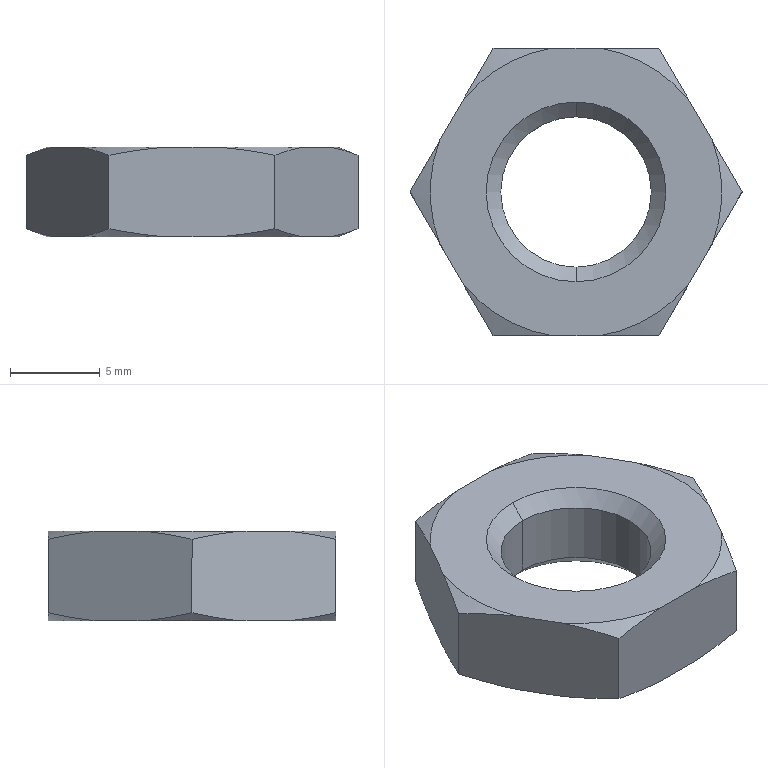Part | STEP file | Microwave Drying Flat Conveyor-nut_iso_4035_-_d_m10_-_05 | 1 solid | 26 faces | box 18.475 x 16 x 5 mm | volume 809.954 mm3 | cone 16 | plane 8 | cylinder 2 | commonest cylinder face diameters 8.376 x2
STEP:
#1=CARTESIAN_POINT('',(0.,-4.188,0.8119));
#2=VERTEX_POINT('',#1);
#3=CARTESIAN_POINT('',(0.,4.188,0.8119));
#4=VERTEX_POINT('',#3);
#5=CARTESIAN_POINT('',(0.,0.,0.8119));
#6=DIRECTION('',(0.,0.,-1.));
#7=DIRECTION('',(0.,1.,0.));
#8=AXIS2_PLACEMENT_3D('',#5,#6,#7);
#9=CIRCLE('',#8,4.188);
#10=EDGE_CURVE('',#2,#4,#9,.T.);
#11=ORIENTED_EDGE('',*,*,#10,.F.);
#12=CARTESIAN_POINT('',(0.,-5.,0.));
#13=VERTEX_POINT('',#12);
#14=CARTESIAN_POINT('',(0.,-4.188,0.8119));
#15=DIRECTION('',(0.,-0.7071,-0.7071));
#16=VECTOR('',#15,1000.);
#17=LINE('',#14,#16);
#18=EDGE_CURVE('',#2,#13,#17,.T.);
#19=ORIENTED_EDGE('',*,*,#18,.T.);
#20=CARTESIAN_POINT('',(0.,5.,0.));
#21=VERTEX_POINT('',#20);
#22=CARTESIAN_POINT('',(0.,0.,0.));
#23=DIRECTION('',(0.,0.,-1.));
#24=DIRECTION('',(1.,0.,0.));
#25=AXIS2_PLACEMENT_3D('',#22,#23,#24);
#26=CIRCLE('',#25,5.);
#27=EDGE_CURVE('',#13,#21,#26,.T.);
#28=ORIENTED_EDGE('',*,*,#27,.T.);
#29=CARTESIAN_POINT('',(0.,4.188,0.8119));
#30=DIRECTION('',(0.,0.7071,-0.7071));
#31=VECTOR('',#30,1000.);
#32=LINE('',#29,#31);
#33=EDGE_CURVE('',#4,#21,#32,.T.);
#34=ORIENTED_EDGE('',*,*,#33,.F.);
#35=EDGE_LOOP('',(#11,#19,#28,#34));
#36=FACE_OUTER_BOUND('',#35,.T.);
#37=CARTESIAN_POINT('',(0.,0.,0.8119));
#38=DIRECTION('',(0.,0.,-1.));
#39=DIRECTION('',(0.,1.,0.));
#40=AXIS2_PLACEMENT_3D('',#37,#38,#39);
#41=CONICAL_SURFACE('',#40,4.188,0.7854);
#42=ADVANCED_FACE('',(#36),#41,.F.);
#43=CARTESIAN_POINT('',(0.,-4.188,4.188));
#44=VERTEX_POINT('',#43);
#45=CARTESIAN_POINT('',(0.,4.188,4.188));
#46=VERTEX_POINT('',#45);
#47=CARTESIAN_POINT('',(0.,0.,4.188));
#48=DIRECTION('',(0.,0.,-1.));
#49=DIRECTION('',(0.,1.,0.));
#50=AXIS2_PLACEMENT_3D('',#47,#48,#49);
#51=CIRCLE('',#50,4.188);
#52=EDGE_CURVE('',#44,#46,#51,.T.);
#53=ORIENTED_EDGE('',*,*,#52,.F.);
#54=CARTESIAN_POINT('',(0.,-4.188,0.));
#55=DIRECTION('',(0.,0.,-1.));
#56=VECTOR('',#55,1000.);
#57=LINE('',#54,#56);
#58=EDGE_CURVE('',#44,#2,#57,.T.);
#59=ORIENTED_EDGE('',*,*,#58,.T.);
#60=ORIENTED_EDGE('',*,*,#10,.T.);
#61=CARTESIAN_POINT('',(0.,4.188,0.));
#62=DIRECTION('',(0.,0.,-1.));
#63=VECTOR('',#62,1000.);
#64=LINE('',#61,#63);
#65=EDGE_CURVE('',#46,#4,#64,.T.);
#66=ORIENTED_EDGE('',*,*,#65,.F.);
#67=EDGE_LOOP('',(#53,#59,#60,#66));
#68=FACE_OUTER_BOUND('',#67,.T.);
#69=CARTESIAN_POINT('',(0.,0.,0.));
#70=DIRECTION('',(0.,0.,-1.));
#71=DIRECTION('',(0.,1.,0.));
#72=AXIS2_PLACEMENT_3D('',#69,#70,#71);
#73=CYLINDRICAL_SURFACE('',#72,4.188);
#74=ADVANCED_FACE('',(#68),#73,.F.);
#75=ORIENTED_EDGE('',*,*,#52,.T.);
#76=CARTESIAN_POINT('',(0.,5.,5.));
#77=VERTEX_POINT('',#76);
#78=CARTESIAN_POINT('',(0.,5.,5.));
#79=DIRECTION('',(0.,0.7071,0.7071));
#80=VECTOR('',#79,1000.);
#81=LINE('',#78,#80);
#82=EDGE_CURVE('',#46,#77,#81,.T.);
#83=ORIENTED_EDGE('',*,*,#82,.T.);
#84=CARTESIAN_POINT('',(0.,-5.,5.));
#85=VERTEX_POINT('',#84);
#86=CARTESIAN_POINT('',(0.,0.,5.));
#87=DIRECTION('',(0.,0.,-1.));
#88=DIRECTION('',(0.,1.,0.));
#89=AXIS2_PLACEMENT_3D('',#86,#87,#88);
#90=CIRCLE('',#89,5.);
#91=EDGE_CURVE('',#85,#77,#90,.T.);
#92=ORIENTED_EDGE('',*,*,#91,.F.);
#93=CARTESIAN_POINT('',(0.,-5.,5.));
#94=DIRECTION('',(0.,-0.7071,0.7071));
#95=VECTOR('',#94,1000.);
#96=LINE('',#93,#95);
#97=EDGE_CURVE('',#44,#85,#96,.T.);
#98=ORIENTED_EDGE('',*,*,#97,.F.);
#99=EDGE_LOOP('',(#75,#83,#92,#98));
#100=FACE_OUTER_BOUND('',#99,.T.);
#101=CARTESIAN_POINT('',(0.,0.,5.));
#102=DIRECTION('',(0.,0.,1.));
#103=DIRECTION('',(0.,-1.,0.));
#104=AXIS2_PLACEMENT_3D('',#101,#102,#103);
#105=CONICAL_SURFACE('',#104,5.,0.7854);
#106=ADVANCED_FACE('',(#100),#105,.F.);
#107=CARTESIAN_POINT('',(7.602,2.834,0.));
#108=VERTEX_POINT('',#107);
#109=CARTESIAN_POINT('',(9.238,0.,0.4545));
#110=VERTEX_POINT('',#109);
#111=CARTESIAN_POINT('',(7.602,2.834,0.));
#112=CARTESIAN_POINT('',(8.152,1.88,0.07388));
#113=CARTESIAN_POINT('',(8.697,0.9365,0.2361));
#114=CARTESIAN_POINT('',(9.238,0.,0.4545));
#115=B_SPLINE_CURVE_WITH_KNOTS('',3,(#111,#112,#113,#114),.UNSPECIFIED.,.F.,.F.,(4,4),(0.00000003,0.003304),.UNSPECIFIED.);
#116=EDGE_CURVE('',#108,#110,#115,.T.);
#117=ORIENTED_EDGE('',*,*,#116,.T.);
#118=CARTESIAN_POINT('',(7.602,-2.834,0.));
#119=VERTEX_POINT('',#118);
#120=CARTESIAN_POINT('',(9.238,0.,0.4545));
#121=CARTESIAN_POINT('',(8.697,-0.9365,0.2361));
#122=CARTESIAN_POINT('',(8.152,-1.88,0.07388));
#123=CARTESIAN_POINT('',(7.602,-2.834,0.));
#124=B_SPLINE_CURVE_WITH_KNOTS('',3,(#120,#121,#122,#123),.UNSPECIFIED.,.F.,.F.,(4,4),(0.000000002,0.003303),.UNSPECIFIED.);
#125=EDGE_CURVE('',#110,#119,#124,.T.);
#126=ORIENTED_EDGE('',*,*,#125,.T.);
#127=CARTESIAN_POINT('',(0.,0.,0.));
#128=DIRECTION('',(0.,0.,1.));
#129=DIRECTION('',(1.,0.,0.));
#130=AXIS2_PLACEMENT_3D('',#127,#128,#129);
#131=CIRCLE('',#130,8.113);
#132=EDGE_CURVE('',#119,#108,#131,.T.);
#133=ORIENTED_EDGE('',*,*,#132,.T.);
#134=EDGE_LOOP('',(#117,#126,#133));
#135=FACE_OUTER_BOUND('',#134,.T.);
#136=CARTESIAN_POINT('',(0.,0.,0.));
#137=DIRECTION('',(0.,0.,1.));
#138=DIRECTION('',(0.,-1.,0.));
#139=AXIS2_PLACEMENT_3D('',#136,#137,#138);
#140=CONICAL_SURFACE('',#139,8.113,1.187);
#141=ADVANCED_FACE('',(#135),#140,.T.);
#142=CARTESIAN_POINT('',(6.255,-5.166,0.));
#143=VERTEX_POINT('',#142);
#144=CARTESIAN_POINT('',(4.619,-8.,0.4545));
#145=VERTEX_POINT('',#144);
#146=CARTESIAN_POINT('',(6.255,-5.166,0.));
#147=CARTESIAN_POINT('',(5.704,-6.12,0.07388));
#148=CARTESIAN_POINT('',(5.159,-7.063,0.2361));
#149=CARTESIAN_POINT('',(4.619,-8.,0.4545));
#150=B_SPLINE_CURVE_WITH_KNOTS('',3,(#146,#147,#148,#149),.UNSPECIFIED.,.F.,.F.,(4,4),(0.00000003,0.003304),.UNSPECIFIED.);
#151=EDGE_CURVE('',#143,#145,#150,.T.);
#152=ORIENTED_EDGE('',*,*,#151,.F.);
#153=CARTESIAN_POINT('',(4.619,-8.,0.));
#154=DIRECTION('',(0.5,0.866,0.));
#155=VECTOR('',#154,1000.);
#156=LINE('',#153,#155);
#157=EDGE_CURVE('',#143,#119,#156,.T.);
#158=ORIENTED_EDGE('',*,*,#157,.T.);
#159=ORIENTED_EDGE('',*,*,#125,.F.);
#160=CARTESIAN_POINT('',(9.238,0.,4.545));
#161=VERTEX_POINT('',#160);
#162=CARTESIAN_POINT('',(9.238,0.,5.));
#163=DIRECTION('',(0.,0.,-1.));
#164=VECTOR('',#163,1000.);
#165=LINE('',#162,#164);
#166=EDGE_CURVE('',#161,#110,#165,.T.);
#167=ORIENTED_EDGE('',*,*,#166,.F.);
#168=CARTESIAN_POINT('',(7.602,-2.834,5.));
#169=VERTEX_POINT('',#168);
#170=CARTESIAN_POINT('',(7.602,-2.834,5.));
#171=CARTESIAN_POINT('',(8.152,-1.88,4.926));
#172=CARTESIAN_POINT('',(8.697,-0.9365,4.764));
#173=CARTESIAN_POINT('',(9.238,0.,4.545));
#174=B_SPLINE_CURVE_WITH_KNOTS('',3,(#170,#171,#172,#173),.UNSPECIFIED.,.F.,.F.,(4,4),(0.00000003,0.003304),.UNSPECIFIED.);
#175=EDGE_CURVE('',#169,#161,#174,.T.);
#176=ORIENTED_EDGE('',*,*,#175,.F.);
#177=CARTESIAN_POINT('',(6.255,-5.166,5.));
#178=VERTEX_POINT('',#177);
#179=CARTESIAN_POINT('',(4.619,-8.,5.));
#180=DIRECTION('',(0.5,0.866,0.));
#181=VECTOR('',#180,1000.);
#182=LINE('',#179,#181);
#183=EDGE_CURVE('',#178,#169,#182,.T.);
#184=ORIENTED_EDGE('',*,*,#183,.F.);
#185=CARTESIAN_POINT('',(4.619,-8.,4.545));
#186=VERTEX_POINT('',#185);
#187=CARTESIAN_POINT('',(4.619,-8.,4.545));
#188=CARTESIAN_POINT('',(5.159,-7.063,4.764));
#189=CARTESIAN_POINT('',(5.704,-6.12,4.926));
#190=CARTESIAN_POINT('',(6.255,-5.166,5.));
#191=B_SPLINE_CURVE_WITH_KNOTS('',3,(#187,#188,#189,#190),.UNSPECIFIED.,.F.,.F.,(4,4),(0.000000002,0.003303),.UNSPECIFIED.);
#192=EDGE_CURVE('',#186,#178,#191,.T.);
#193=ORIENTED_EDGE('',*,*,#192,.F.);
#194=CARTESIAN_POINT('',(4.619,-8.,5.));
#195=DIRECTION('',(0.,0.,-1.));
#196=VECTOR('',#195,1000.);
#197=LINE('',#194,#196);
#198=EDGE_CURVE('',#186,#145,#197,.T.);
#199=ORIENTED_EDGE('',*,*,#198,.T.);
#200=EDGE_LOOP('',(#152,#158,#159,#167,#176,#184,#193,#199));
#201=FACE_OUTER_BOUND('',#200,.T.);
#202=CARTESIAN_POINT('',(4.619,-8.,5.));
#203=DIRECTION('',(-0.866,0.5,0.));
#204=DIRECTION('',(-0.5,-0.866,0.));
#205=AXIS2_PLACEMENT_3D('',#202,#203,#204);
#206=PLANE('',#205);
#207=ADVANCED_FACE('',(#201),#206,.F.);
#208=ORIENTED_EDGE('',*,*,#116,.F.);
#209=CARTESIAN_POINT('',(6.255,5.166,0.));
#210=VERTEX_POINT('',#209);
#211=CARTESIAN_POINT('',(9.238,0.,0.));
#212=DIRECTION('',(-0.5,0.866,0.));
#213=VECTOR('',#212,1000.);
#214=LINE('',#211,#213);
#215=EDGE_CURVE('',#108,#210,#214,.T.);
#216=ORIENTED_EDGE('',*,*,#215,.T.);
#217=CARTESIAN_POINT('',(4.619,8.,0.4545));
#218=VERTEX_POINT('',#217);
#219=CARTESIAN_POINT('',(4.619,8.,0.4545));
#220=CARTESIAN_POINT('',(5.159,7.063,0.2361));
#221=CARTESIAN_POINT('',(5.704,6.12,0.07388));
#222=CARTESIAN_POINT('',(6.255,5.166,0.));
#223=B_SPLINE_CURVE_WITH_KNOTS('',3,(#219,#220,#221,#222),.UNSPECIFIED.,.F.,.F.,(4,4),(0.000000002,0.003303),.UNSPECIFIED.);
#224=EDGE_CURVE('',#218,#210,#223,.T.);
#225=ORIENTED_EDGE('',*,*,#224,.F.);
#226=CARTESIAN_POINT('',(4.619,8.,4.545));
#227=VERTEX_POINT('',#226);
#228=CARTESIAN_POINT('',(4.619,8.,5.));
#229=DIRECTION('',(0.,0.,-1.));
#230=VECTOR('',#229,1000.);
#231=LINE('',#228,#230);
#232=EDGE_CURVE('',#227,#218,#231,.T.);
#233=ORIENTED_EDGE('',*,*,#232,.F.);
#234=CARTESIAN_POINT('',(6.255,5.166,5.));
#235=VERTEX_POINT('',#234);
#236=CARTESIAN_POINT('',(6.255,5.166,5.));
#237=CARTESIAN_POINT('',(5.704,6.12,4.926));
#238=CARTESIAN_POINT('',(5.159,7.063,4.764));
#239=CARTESIAN_POINT('',(4.619,8.,4.545));
#240=B_SPLINE_CURVE_WITH_KNOTS('',3,(#236,#237,#238,#239),.UNSPECIFIED.,.F.,.F.,(4,4),(0.00000003,0.003304),.UNSPECIFIED.);
#241=EDGE_CURVE('',#235,#227,#240,.T.);
#242=ORIENTED_EDGE('',*,*,#241,.F.);
#243=CARTESIAN_POINT('',(7.602,2.834,5.));
#244=VERTEX_POINT('',#243);
#245=CARTESIAN_POINT('',(9.238,0.,5.));
#246=DIRECTION('',(-0.5,0.866,0.));
#247=VECTOR('',#246,1000.);
#248=LINE('',#245,#247);
#249=EDGE_CURVE('',#244,#235,#248,.T.);
#250=ORIENTED_EDGE('',*,*,#249,.F.);
#251=CARTESIAN_POINT('',(9.238,0.,4.545));
#252=CARTESIAN_POINT('',(8.697,0.9365,4.764));
#253=CARTESIAN_POINT('',(8.152,1.88,4.926));
#254=CARTESIAN_POINT('',(7.602,2.834,5.));
#255=B_SPLINE_CURVE_WITH_KNOTS('',3,(#251,#252,#253,#254),.UNSPECIFIED.,.F.,.F.,(4,4),(0.000000002,0.003303),.UNSPECIFIED.);
#256=EDGE_CURVE('',#161,#244,#255,.T.);
#257=ORIENTED_EDGE('',*,*,#256,.F.);
#258=ORIENTED_EDGE('',*,*,#166,.T.);
#259=EDGE_LOOP('',(#208,#216,#225,#233,#242,#250,#257,#258));
#260=FACE_OUTER_BOUND('',#259,.T.);
#261=CARTESIAN_POINT('',(9.238,0.,5.));
#262=DIRECTION('',(-0.866,-0.5,0.));
#263=DIRECTION('',(0.5,-0.866,0.));
#264=AXIS2_PLACEMENT_3D('',#261,#262,#263);
#265=PLANE('',#264);
#266=ADVANCED_FACE('',(#260),#265,.F.);
#267=CARTESIAN_POINT('',(-4.619,8.,0.4545));
#268=VERTEX_POINT('',#267);
#269=CARTESIAN_POINT('',(-1.347,8.,0.));
#270=VERTEX_POINT('',#269);
#271=CARTESIAN_POINT('',(-4.619,8.,0.4545));
#272=CARTESIAN_POINT('',(-4.078,8.,0.3453));
#273=CARTESIAN_POINT('',(-3.532,8.,0.2495));
#274=CARTESIAN_POINT('',(-2.439,8.,0.0951));
#275=CARTESIAN_POINT('',(-1.893,8.,0.03663));
#276=CARTESIAN_POINT('',(-1.347,8.,0.));
#277=B_SPLINE_CURVE_WITH_KNOTS('',3,(#271,#272,#273,#274,#275,#276),.UNSPECIFIED.,.F.,.F.,(4,2,4),(0.007925,0.009576,0.01123),.UNSPECIFIED.);
#278=EDGE_CURVE('',#268,#270,#277,.T.);
#279=ORIENTED_EDGE('',*,*,#278,.F.);
#280=CARTESIAN_POINT('',(-4.619,8.,4.545));
#281=VERTEX_POINT('',#280);
#282=CARTESIAN_POINT('',(-4.619,8.,5.));
#283=DIRECTION('',(0.,0.,-1.));
#284=VECTOR('',#283,1000.);
#285=LINE('',#282,#284);
#286=EDGE_CURVE('',#281,#268,#285,.T.);
#287=ORIENTED_EDGE('',*,*,#286,.F.);
#288=CARTESIAN_POINT('',(-1.347,8.,5.));
#289=VERTEX_POINT('',#288);
#290=CARTESIAN_POINT('',(-1.347,8.,5.));
#291=CARTESIAN_POINT('',(-1.893,8.,4.963));
#292=CARTESIAN_POINT('',(-2.439,8.,4.905));
#293=CARTESIAN_POINT('',(-3.532,8.,4.751));
#294=CARTESIAN_POINT('',(-4.078,8.,4.655));
#295=CARTESIAN_POINT('',(-4.619,8.,4.545));
#296=B_SPLINE_CURVE_WITH_KNOTS('',3,(#290,#291,#292,#293,#294,#295),.UNSPECIFIED.,.F.,.F.,(4,2,4),(0.02193,0.02357,0.02522),.UNSPECIFIED.);
#297=EDGE_CURVE('',#289,#281,#296,.T.);
#298=ORIENTED_EDGE('',*,*,#297,.F.);
#299=CARTESIAN_POINT('',(1.347,8.,5.));
#300=VERTEX_POINT('',#299);
#301=CARTESIAN_POINT('',(4.619,8.,5.));
#302=DIRECTION('',(-1.,0.,0.));
#303=VECTOR('',#302,1000.);
#304=LINE('',#301,#303);
#305=EDGE_CURVE('',#300,#289,#304,.T.);
#306=ORIENTED_EDGE('',*,*,#305,.F.);
#307=CARTESIAN_POINT('',(4.619,8.,4.545));
#308=CARTESIAN_POINT('',(4.078,8.,4.655));
#309=CARTESIAN_POINT('',(3.531,8.,4.751));
#310=CARTESIAN_POINT('',(2.439,8.,4.905));
#311=CARTESIAN_POINT('',(1.893,8.,4.963));
#312=CARTESIAN_POINT('',(1.347,8.,5.));
#313=B_SPLINE_CURVE_WITH_KNOTS('',3,(#307,#308,#309,#310,#311,#312),.UNSPECIFIED.,.F.,.F.,(4,2,4),(0.01593,0.01758,0.01922),.UNSPECIFIED.);
#314=EDGE_CURVE('',#227,#300,#313,.T.);
#315=ORIENTED_EDGE('',*,*,#314,.F.);
#316=ORIENTED_EDGE('',*,*,#232,.T.);
#317=CARTESIAN_POINT('',(1.347,8.,0.));
#318=VERTEX_POINT('',#317);
#319=CARTESIAN_POINT('',(1.347,8.,0.));
#320=CARTESIAN_POINT('',(1.893,8.,0.03664));
#321=CARTESIAN_POINT('',(2.439,8.,0.09509));
#322=CARTESIAN_POINT('',(3.531,8.,0.2494));
#323=CARTESIAN_POINT('',(4.078,8.,0.3453));
#324=CARTESIAN_POINT('',(4.619,8.,0.4545));
#325=B_SPLINE_CURVE_WITH_KNOTS('',3,(#319,#320,#321,#322,#323,#324),.UNSPECIFIED.,.F.,.F.,(4,2,4),(0.01394,0.0156,0.01725),.UNSPECIFIED.);
#326=EDGE_CURVE('',#318,#218,#325,.T.);
#327=ORIENTED_EDGE('',*,*,#326,.F.);
#328=CARTESIAN_POINT('',(4.619,8.,0.));
#329=DIRECTION('',(-1.,0.,0.));
#330=VECTOR('',#329,1000.);
#331=LINE('',#328,#330);
#332=EDGE_CURVE('',#318,#270,#331,.T.);
#333=ORIENTED_EDGE('',*,*,#332,.T.);
#334=EDGE_LOOP('',(#279,#287,#298,#306,#315,#316,#327,#333));
#335=FACE_OUTER_BOUND('',#334,.T.);
#336=CARTESIAN_POINT('',(4.619,8.,5.));
#337=DIRECTION('',(0.,-1.,0.));
#338=DIRECTION('',(1.,0.,0.));
#339=AXIS2_PLACEMENT_3D('',#336,#337,#338);
#340=PLANE('',#339);
#341=ADVANCED_FACE('',(#335),#340,.F.);
#342=CARTESIAN_POINT('',(-6.255,5.166,0.));
#343=VERTEX_POINT('',#342);
#344=CARTESIAN_POINT('',(-6.255,5.166,0.));
#345=CARTESIAN_POINT('',(-5.704,6.12,0.07388));
#346=CARTESIAN_POINT('',(-5.159,7.063,0.2361));
#347=CARTESIAN_POINT('',(-4.619,8.,0.4545));
#348=B_SPLINE_CURVE_WITH_KNOTS('',3,(#344,#345,#346,#347),.UNSPECIFIED.,.F.,.F.,(4,4),(0.00000003,0.003304),.UNSPECIFIED.);
#349=EDGE_CURVE('',#343,#268,#348,.T.);
#350=ORIENTED_EDGE('',*,*,#349,.F.);
#351=CARTESIAN_POINT('',(-7.602,2.834,0.));
#352=VERTEX_POINT('',#351);
#353=CARTESIAN_POINT('',(-4.619,8.,0.));
#354=DIRECTION('',(-0.5,-0.866,0.));
#355=VECTOR('',#354,1000.);
#356=LINE('',#353,#355);
#357=EDGE_CURVE('',#343,#352,#356,.T.);
#358=ORIENTED_EDGE('',*,*,#357,.T.);
#359=CARTESIAN_POINT('',(-9.238,0.,0.4545));
#360=VERTEX_POINT('',#359);
#361=CARTESIAN_POINT('',(-9.238,0.,0.4545));
#362=CARTESIAN_POINT('',(-8.697,0.9365,0.2361));
#363=CARTESIAN_POINT('',(-8.152,1.88,0.07388));
#364=CARTESIAN_POINT('',(-7.602,2.834,0.));
#365=B_SPLINE_CURVE_WITH_KNOTS('',3,(#361,#362,#363,#364),.UNSPECIFIED.,.F.,.F.,(4,4),(0.000000002,0.003303),.UNSPECIFIED.);
#366=EDGE_CURVE('',#360,#352,#365,.T.);
#367=ORIENTED_EDGE('',*,*,#366,.F.);
#368=CARTESIAN_POINT('',(-9.238,0.,4.545));
#369=VERTEX_POINT('',#368);
#370=CARTESIAN_POINT('',(-9.238,0.,5.));
#371=DIRECTION('',(0.,0.,-1.));
#372=VECTOR('',#371,1000.);
#373=LINE('',#370,#372);
#374=EDGE_CURVE('',#369,#360,#373,.T.);
#375=ORIENTED_EDGE('',*,*,#374,.F.);
#376=CARTESIAN_POINT('',(-7.602,2.834,5.));
#377=VERTEX_POINT('',#376);
#378=CARTESIAN_POINT('',(-7.602,2.834,5.));
#379=CARTESIAN_POINT('',(-8.152,1.88,4.926));
#380=CARTESIAN_POINT('',(-8.697,0.9365,4.764));
#381=CARTESIAN_POINT('',(-9.238,0.,4.545));
#382=B_SPLINE_CURVE_WITH_KNOTS('',3,(#378,#379,#380,#381),.UNSPECIFIED.,.F.,.F.,(4,4),(0.00000003,0.003304),.UNSPECIFIED.);
#383=EDGE_CURVE('',#377,#369,#382,.T.);
#384=ORIENTED_EDGE('',*,*,#383,.F.);
#385=CARTESIAN_POINT('',(-6.255,5.166,5.));
#386=VERTEX_POINT('',#385);
#387=CARTESIAN_POINT('',(-4.619,8.,5.));
#388=DIRECTION('',(-0.5,-0.866,0.));
#389=VECTOR('',#388,1000.);
#390=LINE('',#387,#389);
#391=EDGE_CURVE('',#386,#377,#390,.T.);
#392=ORIENTED_EDGE('',*,*,#391,.F.);
#393=CARTESIAN_POINT('',(-4.619,8.,4.545));
#394=CARTESIAN_POINT('',(-5.159,7.063,4.764));
#395=CARTESIAN_POINT('',(-5.704,6.12,4.926));
#396=CARTESIAN_POINT('',(-6.255,5.166,5.));
#397=B_SPLINE_CURVE_WITH_KNOTS('',3,(#393,#394,#395,#396),.UNSPECIFIED.,.F.,.F.,(4,4),(0.000000002,0.003303),.UNSPECIFIED.);
#398=EDGE_CURVE('',#281,#386,#397,.T.);
#399=ORIENTED_EDGE('',*,*,#398,.F.);
#400=ORIENTED_EDGE('',*,*,#286,.T.);
#401=EDGE_LOOP('',(#350,#358,#367,#375,#384,#392,#399,#400));
#402=FACE_OUTER_BOUND('',#401,.T.);
#403=CARTESIAN_POINT('',(-4.619,8.,5.));
#404=DIRECTION('',(0.866,-0.5,0.));
#405=DIRECTION('',(0.5,0.866,0.));
#406=AXIS2_PLACEMENT_3D('',#403,#404,#405);
#407=PLANE('',#406);
#408=ADVANCED_FACE('',(#402),#407,.F.);
#409=CARTESIAN_POINT('',(-7.602,-2.834,0.));
#410=VERTEX_POINT('',#409);
#411=CARTESIAN_POINT('',(-7.602,-2.834,0.));
#412=CARTESIAN_POINT('',(-8.152,-1.88,0.07388));
#413=CARTESIAN_POINT('',(-8.697,-0.9365,0.2361));
#414=CARTESIAN_POINT('',(-9.238,0.,0.4545));
#415=B_SPLINE_CURVE_WITH_KNOTS('',3,(#411,#412,#413,#414),.UNSPECIFIED.,.F.,.F.,(4,4),(0.00000003,0.003304),.UNSPECIFIED.);
#416=EDGE_CURVE('',#410,#360,#415,.T.);
#417=ORIENTED_EDGE('',*,*,#416,.F.);
#418=CARTESIAN_POINT('',(-6.255,-5.166,0.));
#419=VERTEX_POINT('',#418);
#420=CARTESIAN_POINT('',(-9.238,0.,0.));
#421=DIRECTION('',(0.5,-0.866,0.));
#422=VECTOR('',#421,1000.);
#423=LINE('',#420,#422);
#424=EDGE_CURVE('',#410,#419,#423,.T.);
#425=ORIENTED_EDGE('',*,*,#424,.T.);
#426=CARTESIAN_POINT('',(-4.619,-8.,0.4545));
#427=VERTEX_POINT('',#426);
#428=CARTESIAN_POINT('',(-4.619,-8.,0.4545));
#429=CARTESIAN_POINT('',(-5.159,-7.063,0.2361));
#430=CARTESIAN_POINT('',(-5.704,-6.12,0.07388));
#431=CARTESIAN_POINT('',(-6.255,-5.166,0.));
#432=B_SPLINE_CURVE_WITH_KNOTS('',3,(#428,#429,#430,#431),.UNSPECIFIED.,.F.,.F.,(4,4),(0.000000002,0.003303),.UNSPECIFIED.);
#433=EDGE_CURVE('',#427,#419,#432,.T.);
#434=ORIENTED_EDGE('',*,*,#433,.F.);
#435=CARTESIAN_POINT('',(-4.619,-8.,4.545));
#436=VERTEX_POINT('',#435);
#437=CARTESIAN_POINT('',(-4.619,-8.,5.));
#438=DIRECTION('',(0.,0.,-1.));
#439=VECTOR('',#438,1000.);
#440=LINE('',#437,#439);
#441=EDGE_CURVE('',#436,#427,#440,.T.);
#442=ORIENTED_EDGE('',*,*,#441,.F.);
#443=CARTESIAN_POINT('',(-6.255,-5.166,5.));
#444=VERTEX_POINT('',#443);
#445=CARTESIAN_POINT('',(-6.255,-5.166,5.));
#446=CARTESIAN_POINT('',(-5.704,-6.12,4.926));
#447=CARTESIAN_POINT('',(-5.159,-7.063,4.764));
#448=CARTESIAN_POINT('',(-4.619,-8.,4.545));
#449=B_SPLINE_CURVE_WITH_KNOTS('',3,(#445,#446,#447,#448),.UNSPECIFIED.,.F.,.F.,(4,4),(0.00000003,0.003304),.UNSPECIFIED.);
#450=EDGE_CURVE('',#444,#436,#449,.T.);
#451=ORIENTED_EDGE('',*,*,#450,.F.);
#452=CARTESIAN_POINT('',(-7.602,-2.834,5.));
#453=VERTEX_POINT('',#452);
#454=CARTESIAN_POINT('',(-9.238,0.,5.));
#455=DIRECTION('',(0.5,-0.866,0.));
#456=VECTOR('',#455,1000.);
#457=LINE('',#454,#456);
#458=EDGE_CURVE('',#453,#444,#457,.T.);
#459=ORIENTED_EDGE('',*,*,#458,.F.);
#460=CARTESIAN_POINT('',(-9.238,0.,4.545));
#461=CARTESIAN_POINT('',(-8.697,-0.9365,4.764));
#462=CARTESIAN_POINT('',(-8.152,-1.88,4.926));
#463=CARTESIAN_POINT('',(-7.602,-2.834,5.));
#464=B_SPLINE_CURVE_WITH_KNOTS('',3,(#460,#461,#462,#463),.UNSPECIFIED.,.F.,.F.,(4,4),(0.000000002,0.003303),.UNSPECIFIED.);
#465=EDGE_CURVE('',#369,#453,#464,.T.);
#466=ORIENTED_EDGE('',*,*,#465,.F.);
#467=ORIENTED_EDGE('',*,*,#374,.T.);
#468=EDGE_LOOP('',(#417,#425,#434,#442,#451,#459,#466,#467));
#469=FACE_OUTER_BOUND('',#468,.T.);
#470=CARTESIAN_POINT('',(-9.238,0.,5.));
#471=DIRECTION('',(0.866,0.5,0.));
#472=DIRECTION('',(-0.5,0.866,0.));
#473=AXIS2_PLACEMENT_3D('',#470,#471,#472);
#474=PLANE('',#473);
#475=ADVANCED_FACE('',(#469),#474,.F.);
#476=CARTESIAN_POINT('',(1.347,-8.,0.));
#477=VERTEX_POINT('',#476);
#478=CARTESIAN_POINT('',(4.619,-8.,0.4545));
#479=CARTESIAN_POINT('',(4.078,-8.,0.3453));
#480=CARTESIAN_POINT('',(3.531,-8.,0.2494));
#481=CARTESIAN_POINT('',(2.439,-8.,0.09509));
#482=CARTESIAN_POINT('',(1.893,-8.,0.03664));
#483=CARTESIAN_POINT('',(1.347,-8.,0.));
#484=B_SPLINE_CURVE_WITH_KNOTS('',3,(#478,#479,#480,#481,#482,#483),.UNSPECIFIED.,.F.,.F.,(4,2,4),(0.01593,0.01758,0.01922),.UNSPECIFIED.);
#485=EDGE_CURVE('',#145,#477,#484,.T.);
#486=ORIENTED_EDGE('',*,*,#485,.F.);
#487=ORIENTED_EDGE('',*,*,#198,.F.);
#488=CARTESIAN_POINT('',(1.347,-8.,5.));
#489=VERTEX_POINT('',#488);
#490=CARTESIAN_POINT('',(1.347,-8.,5.));
#491=CARTESIAN_POINT('',(1.893,-8.,4.963));
#492=CARTESIAN_POINT('',(2.439,-8.,4.905));
#493=CARTESIAN_POINT('',(3.531,-8.,4.751));
#494=CARTESIAN_POINT('',(4.078,-8.,4.655));
#495=CARTESIAN_POINT('',(4.619,-8.,4.545));
#496=B_SPLINE_CURVE_WITH_KNOTS('',3,(#490,#491,#492,#493,#494,#495),.UNSPECIFIED.,.F.,.F.,(4,2,4),(0.01394,0.0156,0.01725),.UNSPECIFIED.);
#497=EDGE_CURVE('',#489,#186,#496,.T.);
#498=ORIENTED_EDGE('',*,*,#497,.F.);
#499=CARTESIAN_POINT('',(-1.347,-8.,5.));
#500=VERTEX_POINT('',#499);
#501=CARTESIAN_POINT('',(-4.619,-8.,5.));
#502=DIRECTION('',(1.,0.,0.));
#503=VECTOR('',#502,1000.);
#504=LINE('',#501,#503);
#505=EDGE_CURVE('',#500,#489,#504,.T.);
#506=ORIENTED_EDGE('',*,*,#505,.F.);
#507=CARTESIAN_POINT('',(-4.619,-8.,4.545));
#508=CARTESIAN_POINT('',(-4.078,-8.,4.655));
#509=CARTESIAN_POINT('',(-3.532,-8.,4.751));
#510=CARTESIAN_POINT('',(-2.439,-8.,4.905));
#511=CARTESIAN_POINT('',(-1.893,-8.,4.963));
#512=CARTESIAN_POINT('',(-1.347,-8.,5.));
#513=B_SPLINE_CURVE_WITH_KNOTS('',3,(#507,#508,#509,#510,#511,#512),.UNSPECIFIED.,.F.,.F.,(4,2,4),(0.007925,0.009576,0.01123),.UNSPECIFIED.);
#514=EDGE_CURVE('',#436,#500,#513,.T.);
#515=ORIENTED_EDGE('',*,*,#514,.F.);
#516=ORIENTED_EDGE('',*,*,#441,.T.);
#517=CARTESIAN_POINT('',(-1.347,-8.,0.));
#518=VERTEX_POINT('',#517);
#519=CARTESIAN_POINT('',(-1.347,-8.,0.));
#520=CARTESIAN_POINT('',(-1.893,-8.,0.03663));
#521=CARTESIAN_POINT('',(-2.439,-8.,0.0951));
#522=CARTESIAN_POINT('',(-3.532,-8.,0.2495));
#523=CARTESIAN_POINT('',(-4.078,-8.,0.3453));
#524=CARTESIAN_POINT('',(-4.619,-8.,0.4545));
#525=B_SPLINE_CURVE_WITH_KNOTS('',3,(#519,#520,#521,#522,#523,#524),.UNSPECIFIED.,.F.,.F.,(4,2,4),(0.02193,0.02357,0.02522),.UNSPECIFIED.);
#526=EDGE_CURVE('',#518,#427,#525,.T.);
#527=ORIENTED_EDGE('',*,*,#526,.F.);
#528=CARTESIAN_POINT('',(-4.619,-8.,0.));
#529=DIRECTION('',(1.,0.,0.));
#530=VECTOR('',#529,1000.);
#531=LINE('',#528,#530);
#532=EDGE_CURVE('',#518,#477,#531,.T.);
#533=ORIENTED_EDGE('',*,*,#532,.T.);
#534=EDGE_LOOP('',(#486,#487,#498,#506,#515,#516,#527,#533));
#535=FACE_OUTER_BOUND('',#534,.T.);
#536=CARTESIAN_POINT('',(-4.619,-8.,5.));
#537=DIRECTION('',(0.,1.,0.));
#538=DIRECTION('',(-1.,0.,0.));
#539=AXIS2_PLACEMENT_3D('',#536,#537,#538);
#540=PLANE('',#539);
#541=ADVANCED_FACE('',(#535),#540,.F.);
#542=ORIENTED_EDGE('',*,*,#91,.T.);
#543=CARTESIAN_POINT('',(0.,0.,5.));
#544=DIRECTION('',(0.,0.,-1.));
#545=DIRECTION('',(0.,1.,0.));
#546=AXIS2_PLACEMENT_3D('',#543,#544,#545);
#547=CIRCLE('',#546,5.);
#548=EDGE_CURVE('',#77,#85,#547,.T.);
#549=ORIENTED_EDGE('',*,*,#548,.T.);
#550=EDGE_LOOP('',(#542,#549));
#551=FACE_BOUND('',#550,.T.);
#552=ORIENTED_EDGE('',*,*,#249,.T.);
#553=CARTESIAN_POINT('',(0.,0.,5.));
#554=DIRECTION('',(0.,0.,-1.));
#555=DIRECTION('',(0.,1.,0.));
#556=AXIS2_PLACEMENT_3D('',#553,#554,#555);
#557=CIRCLE('',#556,8.113);
#558=EDGE_CURVE('',#300,#235,#557,.T.);
#559=ORIENTED_EDGE('',*,*,#558,.F.);
#560=ORIENTED_EDGE('',*,*,#305,.T.);
#561=CARTESIAN_POINT('',(0.,0.,5.));
#562=DIRECTION('',(0.,0.,1.));
#563=DIRECTION('',(1.,0.,0.));
#564=AXIS2_PLACEMENT_3D('',#561,#562,#563);
#565=CIRCLE('',#564,8.113);
#566=EDGE_CURVE('',#289,#386,#565,.T.);
#567=ORIENTED_EDGE('',*,*,#566,.T.);
#568=ORIENTED_EDGE('',*,*,#391,.T.);
#569=CARTESIAN_POINT('',(0.,0.,5.));
#570=DIRECTION('',(0.,0.,1.));
#571=DIRECTION('',(1.,0.,0.));
#572=AXIS2_PLACEMENT_3D('',#569,#570,#571);
#573=CIRCLE('',#572,8.113);
#574=EDGE_CURVE('',#377,#453,#573,.T.);
#575=ORIENTED_EDGE('',*,*,#574,.T.);
#576=ORIENTED_EDGE('',*,*,#458,.T.);
#577=CARTESIAN_POINT('',(0.,0.,5.));
#578=DIRECTION('',(0.,0.,1.));
#579=DIRECTION('',(1.,0.,0.));
#580=AXIS2_PLACEMENT_3D('',#577,#578,#579);
#581=CIRCLE('',#580,8.113);
#582=EDGE_CURVE('',#444,#500,#581,.T.);
#583=ORIENTED_EDGE('',*,*,#582,.T.);
#584=ORIENTED_EDGE('',*,*,#505,.T.);
#585=CARTESIAN_POINT('',(0.,0.,5.));
#586=DIRECTION('',(0.,0.,1.));
#587=DIRECTION('',(1.,0.,0.));
#588=AXIS2_PLACEMENT_3D('',#585,#586,#587);
#589=CIRCLE('',#588,8.113);
#590=EDGE_CURVE('',#489,#178,#589,.T.);
#591=ORIENTED_EDGE('',*,*,#590,.T.);
#592=ORIENTED_EDGE('',*,*,#183,.T.);
#593=CARTESIAN_POINT('',(0.,0.,5.));
#594=DIRECTION('',(0.,0.,1.));
#595=DIRECTION('',(1.,0.,0.));
#596=AXIS2_PLACEMENT_3D('',#593,#594,#595);
#597=CIRCLE('',#596,8.113);
#598=EDGE_CURVE('',#169,#244,#597,.T.);
#599=ORIENTED_EDGE('',*,*,#598,.T.);
#600=EDGE_LOOP('',(#552,#559,#560,#567,#568,#575,#576,#583,#584,#591,#592,#599));
#601=FACE_OUTER_BOUND('',#600,.T.);
#602=CARTESIAN_POINT('',(9.238,0.,5.));
#603=DIRECTION('',(0.,0.,1.));
#604=DIRECTION('',(1.,0.,0.));
#605=AXIS2_PLACEMENT_3D('',#602,#603,#604);
#606=PLANE('',#605);
#607=ADVANCED_FACE('',(#551,#601),#606,.T.);
#608=CARTESIAN_POINT('',(0.,0.,0.));
#609=DIRECTION('',(0.,0.,-1.));
#610=DIRECTION('',(1.,0.,0.));
#611=AXIS2_PLACEMENT_3D('',#608,#609,#610);
#612=CIRCLE('',#611,5.);
#613=EDGE_CURVE('',#21,#13,#612,.T.);
#614=ORIENTED_EDGE('',*,*,#613,.F.);
#615=ORIENTED_EDGE('',*,*,#27,.F.);
#616=EDGE_LOOP('',(#614,#615));
#617=FACE_BOUND('',#616,.T.);
#618=CARTESIAN_POINT('',(0.,0.,0.));
#619=DIRECTION('',(0.,0.,-1.));
#620=DIRECTION('',(0.,1.,0.));
#621=AXIS2_PLACEMENT_3D('',#618,#619,#620);
#622=CIRCLE('',#621,8.113);
#623=EDGE_CURVE('',#318,#210,#622,.T.);
#624=ORIENTED_EDGE('',*,*,#623,.T.);
#625=ORIENTED_EDGE('',*,*,#215,.F.);
#626=ORIENTED_EDGE('',*,*,#132,.F.);
#627=ORIENTED_EDGE('',*,*,#157,.F.);
#628=CARTESIAN_POINT('',(0.,0.,0.));
#629=DIRECTION('',(0.,0.,1.));
#630=DIRECTION('',(1.,0.,0.));
#631=AXIS2_PLACEMENT_3D('',#628,#629,#630);
#632=CIRCLE('',#631,8.113);
#633=EDGE_CURVE('',#477,#143,#632,.T.);
#634=ORIENTED_EDGE('',*,*,#633,.F.);
#635=ORIENTED_EDGE('',*,*,#532,.F.);
#636=CARTESIAN_POINT('',(0.,0.,0.));
#637=DIRECTION('',(0.,0.,1.));
#638=DIRECTION('',(1.,0.,0.));
#639=AXIS2_PLACEMENT_3D('',#636,#637,#638);
#640=CIRCLE('',#639,8.113);
#641=EDGE_CURVE('',#419,#518,#640,.T.);
#642=ORIENTED_EDGE('',*,*,#641,.F.);
#643=ORIENTED_EDGE('',*,*,#424,.F.);
#644=CARTESIAN_POINT('',(0.,0.,0.));
#645=DIRECTION('',(0.,0.,1.));
#646=DIRECTION('',(1.,0.,0.));
#647=AXIS2_PLACEMENT_3D('',#644,#645,#646);
#648=CIRCLE('',#647,8.113);
#649=EDGE_CURVE('',#352,#410,#648,.T.);
#650=ORIENTED_EDGE('',*,*,#649,.F.);
#651=ORIENTED_EDGE('',*,*,#357,.F.);
#652=CARTESIAN_POINT('',(0.,0.,0.));
#653=DIRECTION('',(0.,0.,1.));
#654=DIRECTION('',(1.,0.,0.));
#655=AXIS2_PLACEMENT_3D('',#652,#653,#654);
#656=CIRCLE('',#655,8.113);
#657=EDGE_CURVE('',#270,#343,#656,.T.);
#658=ORIENTED_EDGE('',*,*,#657,.F.);
#659=ORIENTED_EDGE('',*,*,#332,.F.);
#660=EDGE_LOOP('',(#624,#625,#626,#627,#634,#635,#642,#643,#650,#651,#658,#659));
#661=FACE_OUTER_BOUND('',#660,.T.);
#662=CARTESIAN_POINT('',(9.238,0.,0.));
#663=DIRECTION('',(0.,0.,1.));
#664=DIRECTION('',(1.,0.,0.));
#665=AXIS2_PLACEMENT_3D('',#662,#663,#664);
#666=PLANE('',#665);
#667=ADVANCED_FACE('',(#617,#661),#666,.F.);
#668=ORIENTED_EDGE('',*,*,#633,.T.);
#669=ORIENTED_EDGE('',*,*,#151,.T.);
#670=ORIENTED_EDGE('',*,*,#485,.T.);
#671=EDGE_LOOP('',(#668,#669,#670));
#672=FACE_OUTER_BOUND('',#671,.T.);
#673=CARTESIAN_POINT('',(0.,0.,0.));
#674=DIRECTION('',(0.,0.,1.));
#675=DIRECTION('',(0.,-1.,0.));
#676=AXIS2_PLACEMENT_3D('',#673,#674,#675);
#677=CONICAL_SURFACE('',#676,8.113,1.187);
#678=ADVANCED_FACE('',(#672),#677,.T.);
#679=ORIENTED_EDGE('',*,*,#526,.T.);
#680=ORIENTED_EDGE('',*,*,#433,.T.);
#681=ORIENTED_EDGE('',*,*,#641,.T.);
#682=EDGE_LOOP('',(#679,#680,#681));
#683=FACE_OUTER_BOUND('',#682,.T.);
#684=CARTESIAN_POINT('',(0.,0.,0.));
#685=DIRECTION('',(0.,0.,1.));
#686=DIRECTION('',(0.,-1.,0.));
#687=AXIS2_PLACEMENT_3D('',#684,#685,#686);
#688=CONICAL_SURFACE('',#687,8.113,1.187);
#689=ADVANCED_FACE('',(#683),#688,.T.);
#690=ORIENTED_EDGE('',*,*,#416,.T.);
#691=ORIENTED_EDGE('',*,*,#366,.T.);
#692=ORIENTED_EDGE('',*,*,#649,.T.);
#693=EDGE_LOOP('',(#690,#691,#692));
#694=FACE_OUTER_BOUND('',#693,.T.);
#695=CARTESIAN_POINT('',(0.,0.,0.));
#696=DIRECTION('',(0.,0.,1.));
#697=DIRECTION('',(0.,-1.,0.));
#698=AXIS2_PLACEMENT_3D('',#695,#696,#697);
#699=CONICAL_SURFACE('',#698,8.113,1.187);
#700=ADVANCED_FACE('',(#694),#699,.T.);
#701=ORIENTED_EDGE('',*,*,#349,.T.);
#702=ORIENTED_EDGE('',*,*,#278,.T.);
#703=ORIENTED_EDGE('',*,*,#657,.T.);
#704=EDGE_LOOP('',(#701,#702,#703));
#705=FACE_OUTER_BOUND('',#704,.T.);
#706=CARTESIAN_POINT('',(0.,0.,0.));
#707=DIRECTION('',(0.,0.,1.));
#708=DIRECTION('',(0.,-1.,0.));
#709=AXIS2_PLACEMENT_3D('',#706,#707,#708);
#710=CONICAL_SURFACE('',#709,8.113,1.187);
#711=ADVANCED_FACE('',(#705),#710,.T.);
#712=ORIENTED_EDGE('',*,*,#326,.T.);
#713=ORIENTED_EDGE('',*,*,#224,.T.);
#714=ORIENTED_EDGE('',*,*,#623,.F.);
#715=EDGE_LOOP('',(#712,#713,#714));
#716=FACE_OUTER_BOUND('',#715,.T.);
#717=CARTESIAN_POINT('',(0.,0.,0.));
#718=DIRECTION('',(0.,0.,1.));
#719=DIRECTION('',(0.,-1.,0.));
#720=AXIS2_PLACEMENT_3D('',#717,#718,#719);
#721=CONICAL_SURFACE('',#720,8.113,1.187);
#722=ADVANCED_FACE('',(#716),#721,.T.);
#723=ORIENTED_EDGE('',*,*,#82,.F.);
#724=CARTESIAN_POINT('',(0.,0.,4.188));
#725=DIRECTION('',(0.,0.,-1.));
#726=DIRECTION('',(0.,1.,0.));
#727=AXIS2_PLACEMENT_3D('',#724,#725,#726);
#728=CIRCLE('',#727,4.188);
#729=EDGE_CURVE('',#46,#44,#728,.T.);
#730=ORIENTED_EDGE('',*,*,#729,.T.);
#731=ORIENTED_EDGE('',*,*,#97,.T.);
#732=ORIENTED_EDGE('',*,*,#548,.F.);
#733=EDGE_LOOP('',(#723,#730,#731,#732));
#734=FACE_OUTER_BOUND('',#733,.T.);
#735=CARTESIAN_POINT('',(0.,0.,5.));
#736=DIRECTION('',(0.,0.,1.));
#737=DIRECTION('',(0.,-1.,0.));
#738=AXIS2_PLACEMENT_3D('',#735,#736,#737);
#739=CONICAL_SURFACE('',#738,5.,0.7854);
#740=ADVANCED_FACE('',(#734),#739,.F.);
#741=ORIENTED_EDGE('',*,*,#58,.F.);
#742=ORIENTED_EDGE('',*,*,#729,.F.);
#743=ORIENTED_EDGE('',*,*,#65,.T.);
#744=CARTESIAN_POINT('',(0.,0.,0.8119));
#745=DIRECTION('',(0.,0.,-1.));
#746=DIRECTION('',(0.,1.,0.));
#747=AXIS2_PLACEMENT_3D('',#744,#745,#746);
#748=CIRCLE('',#747,4.188);
#749=EDGE_CURVE('',#4,#2,#748,.T.);
#750=ORIENTED_EDGE('',*,*,#749,.T.);
#751=EDGE_LOOP('',(#741,#742,#743,#750));
#752=FACE_OUTER_BOUND('',#751,.T.);
#753=CARTESIAN_POINT('',(0.,0.,0.));
#754=DIRECTION('',(0.,0.,-1.));
#755=DIRECTION('',(0.,1.,0.));
#756=AXIS2_PLACEMENT_3D('',#753,#754,#755);
#757=CYLINDRICAL_SURFACE('',#756,4.188);
#758=ADVANCED_FACE('',(#752),#757,.F.);
#759=ORIENTED_EDGE('',*,*,#18,.F.);
#760=ORIENTED_EDGE('',*,*,#749,.F.);
#761=ORIENTED_EDGE('',*,*,#33,.T.);
#762=ORIENTED_EDGE('',*,*,#613,.T.);
#763=EDGE_LOOP('',(#759,#760,#761,#762));
#764=FACE_OUTER_BOUND('',#763,.T.);
#765=CARTESIAN_POINT('',(0.,0.,0.8119));
#766=DIRECTION('',(0.,0.,-1.));
#767=DIRECTION('',(0.,1.,0.));
#768=AXIS2_PLACEMENT_3D('',#765,#766,#767);
#769=CONICAL_SURFACE('',#768,4.188,0.7854);
#770=ADVANCED_FACE('',(#764),#769,.F.);
#771=ORIENTED_EDGE('',*,*,#598,.F.);
#772=ORIENTED_EDGE('',*,*,#175,.T.);
#773=ORIENTED_EDGE('',*,*,#256,.T.);
#774=EDGE_LOOP('',(#771,#772,#773));
#775=FACE_OUTER_BOUND('',#774,.T.);
#776=CARTESIAN_POINT('',(0.,0.,4.545));
#777=DIRECTION('',(0.,0.,-1.));
#778=DIRECTION('',(0.,1.,0.));
#779=AXIS2_PLACEMENT_3D('',#776,#777,#778);
#780=CONICAL_SURFACE('',#779,9.238,1.187);
#781=ADVANCED_FACE('',(#775),#780,.T.);
#782=ORIENTED_EDGE('',*,*,#497,.T.);
#783=ORIENTED_EDGE('',*,*,#192,.T.);
#784=ORIENTED_EDGE('',*,*,#590,.F.);
#785=EDGE_LOOP('',(#782,#783,#784));
#786=FACE_OUTER_BOUND('',#785,.T.);
#787=CARTESIAN_POINT('',(0.,0.,4.545));
#788=DIRECTION('',(0.,0.,-1.));
#789=DIRECTION('',(0.,1.,0.));
#790=AXIS2_PLACEMENT_3D('',#787,#788,#789);
#791=CONICAL_SURFACE('',#790,9.238,1.187);
#792=ADVANCED_FACE('',(#786),#791,.T.);
#793=ORIENTED_EDGE('',*,*,#582,.F.);
#794=ORIENTED_EDGE('',*,*,#450,.T.);
#795=ORIENTED_EDGE('',*,*,#514,.T.);
#796=EDGE_LOOP('',(#793,#794,#795));
#797=FACE_OUTER_BOUND('',#796,.T.);
#798=CARTESIAN_POINT('',(0.,0.,4.545));
#799=DIRECTION('',(0.,0.,-1.));
#800=DIRECTION('',(0.,1.,0.));
#801=AXIS2_PLACEMENT_3D('',#798,#799,#800);
#802=CONICAL_SURFACE('',#801,9.238,1.187);
#803=ADVANCED_FACE('',(#797),#802,.T.);
#804=ORIENTED_EDGE('',*,*,#574,.F.);
#805=ORIENTED_EDGE('',*,*,#383,.T.);
#806=ORIENTED_EDGE('',*,*,#465,.T.);
#807=EDGE_LOOP('',(#804,#805,#806));
#808=FACE_OUTER_BOUND('',#807,.T.);
#809=CARTESIAN_POINT('',(0.,0.,4.545));
#810=DIRECTION('',(0.,0.,-1.));
#811=DIRECTION('',(0.,1.,0.));
#812=AXIS2_PLACEMENT_3D('',#809,#810,#811);
#813=CONICAL_SURFACE('',#812,9.238,1.187);
#814=ADVANCED_FACE('',(#808),#813,.T.);
#815=ORIENTED_EDGE('',*,*,#566,.F.);
#816=ORIENTED_EDGE('',*,*,#297,.T.);
#817=ORIENTED_EDGE('',*,*,#398,.T.);
#818=EDGE_LOOP('',(#815,#816,#817));
#819=FACE_OUTER_BOUND('',#818,.T.);
#820=CARTESIAN_POINT('',(0.,0.,4.545));
#821=DIRECTION('',(0.,0.,-1.));
#822=DIRECTION('',(0.,1.,0.));
#823=AXIS2_PLACEMENT_3D('',#820,#821,#822);
#824=CONICAL_SURFACE('',#823,9.238,1.187);
#825=ADVANCED_FACE('',(#819),#824,.T.);
#826=ORIENTED_EDGE('',*,*,#558,.T.);
#827=ORIENTED_EDGE('',*,*,#241,.T.);
#828=ORIENTED_EDGE('',*,*,#314,.T.);
#829=EDGE_LOOP('',(#826,#827,#828));
#830=FACE_OUTER_BOUND('',#829,.T.);
#831=CARTESIAN_POINT('',(0.,0.,4.545));
#832=DIRECTION('',(0.,0.,-1.));
#833=DIRECTION('',(0.,1.,0.));
#834=AXIS2_PLACEMENT_3D('',#831,#832,#833);
#835=CONICAL_SURFACE('',#834,9.238,1.187);
#836=ADVANCED_FACE('',(#830),#835,.T.);
#837=CLOSED_SHELL('',(#42,#74,#106,#141,#207,#266,#341,#408,#475,#541,#607,#667,#678,#689,#700,#711,#722,#740,#758,#770,#781,#792,#803,#814,#825,#836));
#838=MANIFOLD_SOLID_BREP('',#837);
#839=CARTESIAN_POINT('',(0.,0.,0.));
#840=DIRECTION('',(0.,0.,1.));
#841=DIRECTION('',(1.,0.,0.));
#842=AXIS2_PLACEMENT_3D('',#839,#840,#841);
#843=(LENGTH_UNIT()NAMED_UNIT(*)SI_UNIT(.MILLI.,.METRE.));
#844=UNCERTAINTY_MEASURE_WITH_UNIT(LENGTH_MEASURE(0.00001),#843,'','');
#845=(NAMED_UNIT(*)PLANE_ANGLE_UNIT()SI_UNIT($,.RADIAN.));
#846=(NAMED_UNIT(*)SI_UNIT($,.STERADIAN.)SOLID_ANGLE_UNIT());
#847=(GEOMETRIC_REPRESENTATION_CONTEXT(3)GLOBAL_UNCERTAINTY_ASSIGNED_CONTEXT((#844))GLOBAL_UNIT_ASSIGNED_CONTEXT((#843,#845,#846))REPRESENTATION_CONTEXT('',''));
#848=ADVANCED_BREP_SHAPE_REPRESENTATION('',(#838,#842),#847);